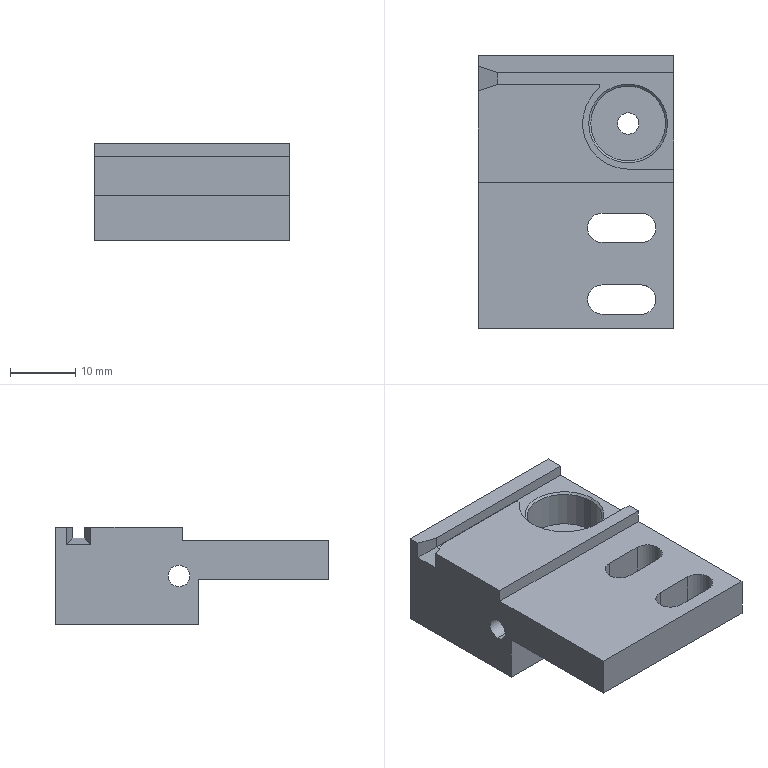Part | NX | features BREP 1 | 1 solid | 39 faces | box 30 x 42 x 15 mm | volume 11527 mm3 | plane 24 | cylinder 13 | cone 2 | commonest cylinder face diameters 4.5 x6 3.3 x4 11.5 x2 14 x1
STEP:
#1=CARTESIAN_POINT('',(-6.05,0.,5.8));
#2=VERTEX_POINT('',#1);
#3=CARTESIAN_POINT('',(-5.75,0.,5.5));
#4=VERTEX_POINT('',#3);
#5=CARTESIAN_POINT('',(-5.75,0.,5.5));
#6=DIRECTION('',(-0.7071,0.,0.7071));
#7=VECTOR('',#6,1000.);
#8=LINE('',#5,#7);
#9=EDGE_CURVE('',#2,#4,#8,.F.);
#10=ORIENTED_EDGE('',*,*,#9,.T.);
#11=CARTESIAN_POINT('',(5.75,0.,5.5));
#12=VERTEX_POINT('',#11);
#13=CARTESIAN_POINT('',(0.,0.,5.5));
#14=DIRECTION('',(0.,0.,1.));
#15=DIRECTION('',(1.,0.,0.));
#16=AXIS2_PLACEMENT_3D('',#13,#14,#15);
#17=CIRCLE('',#16,5.75);
#18=EDGE_CURVE('',#12,#4,#17,.T.);
#19=ORIENTED_EDGE('',*,*,#18,.F.);
#20=CARTESIAN_POINT('',(6.05,0.,5.8));
#21=VERTEX_POINT('',#20);
#22=CARTESIAN_POINT('',(5.75,0.,5.5));
#23=DIRECTION('',(0.7071,0.,0.7071));
#24=VECTOR('',#23,1000.);
#25=LINE('',#22,#24);
#26=EDGE_CURVE('',#21,#12,#25,.F.);
#27=ORIENTED_EDGE('',*,*,#26,.F.);
#28=CARTESIAN_POINT('',(0.,0.,5.8));
#29=DIRECTION('',(0.,0.,-1.));
#30=DIRECTION('',(1.,0.,0.));
#31=AXIS2_PLACEMENT_3D('',#28,#29,#30);
#32=CIRCLE('',#31,6.05);
#33=EDGE_CURVE('',#2,#21,#32,.T.);
#34=ORIENTED_EDGE('',*,*,#33,.F.);
#35=EDGE_LOOP('',(#10,#19,#27,#34));
#36=FACE_BOUND('',#35,.T.);
#37=CARTESIAN_POINT('',(0.,0.,5.5));
#38=DIRECTION('',(0.,0.,1.));
#39=DIRECTION('',(1.,0.,0.));
#40=AXIS2_PLACEMENT_3D('',#37,#38,#39);
#41=CONICAL_SURFACE('',#40,5.75,0.7854);
#42=ADVANCED_FACE('',(#36),#41,.F.);
#43=CARTESIAN_POINT('',(7.,-9.,7.5));
#44=VERTEX_POINT('',#43);
#45=CARTESIAN_POINT('',(-23.,-9.,7.5));
#46=VERTEX_POINT('',#45);
#47=CARTESIAN_POINT('',(-23.,-9.,7.5));
#48=DIRECTION('',(-1.,0.,0.));
#49=VECTOR('',#48,1000.);
#50=LINE('',#47,#49);
#51=EDGE_CURVE('',#44,#46,#50,.T.);
#52=ORIENTED_EDGE('',*,*,#51,.T.);
#53=CARTESIAN_POINT('',(-23.,-9.,5.5));
#54=VERTEX_POINT('',#53);
#55=CARTESIAN_POINT('',(-23.,-9.,5.5));
#56=DIRECTION('',(0.,0.,1.));
#57=VECTOR('',#56,1000.);
#58=LINE('',#55,#57);
#59=EDGE_CURVE('',#54,#46,#58,.T.);
#60=ORIENTED_EDGE('',*,*,#59,.F.);
#61=CARTESIAN_POINT('',(7.,-9.,5.5));
#62=VERTEX_POINT('',#61);
#63=CARTESIAN_POINT('',(-23.,-9.,5.5));
#64=DIRECTION('',(-1.,0.,0.));
#65=VECTOR('',#64,1000.);
#66=LINE('',#63,#65);
#67=EDGE_CURVE('',#62,#54,#66,.T.);
#68=ORIENTED_EDGE('',*,*,#67,.F.);
#69=CARTESIAN_POINT('',(7.,-9.,5.5));
#70=DIRECTION('',(0.,0.,1.));
#71=VECTOR('',#70,1000.);
#72=LINE('',#69,#71);
#73=EDGE_CURVE('',#62,#44,#72,.T.);
#74=ORIENTED_EDGE('',*,*,#73,.T.);
#75=EDGE_LOOP('',(#52,#60,#68,#74));
#76=FACE_BOUND('',#75,.T.);
#77=CARTESIAN_POINT('',(-23.,-9.,5.5));
#78=DIRECTION('',(0.,1.,0.));
#79=DIRECTION('',(0.,0.,1.));
#80=AXIS2_PLACEMENT_3D('',#77,#78,#79);
#81=PLANE('',#80);
#82=ADVANCED_FACE('',(#76),#81,.F.);
#83=CARTESIAN_POINT('',(-4.,-18.25,5.5));
#84=VERTEX_POINT('',#83);
#85=CARTESIAN_POINT('',(-4.,-13.75,5.5));
#86=VERTEX_POINT('',#85);
#87=CARTESIAN_POINT('',(-4.,-16.,5.5));
#88=DIRECTION('',(0.,0.,-1.));
#89=DIRECTION('',(1.,0.,0.));
#90=AXIS2_PLACEMENT_3D('',#87,#88,#89);
#91=CIRCLE('',#90,2.25);
#92=EDGE_CURVE('',#84,#86,#91,.T.);
#93=ORIENTED_EDGE('',*,*,#92,.T.);
#94=CARTESIAN_POINT('',(2.,-13.75,5.5));
#95=VERTEX_POINT('',#94);
#96=CARTESIAN_POINT('',(-4.,-13.75,5.5));
#97=DIRECTION('',(1.,0.,0.));
#98=VECTOR('',#97,1000.);
#99=LINE('',#96,#98);
#100=EDGE_CURVE('',#86,#95,#99,.T.);
#101=ORIENTED_EDGE('',*,*,#100,.T.);
#102=CARTESIAN_POINT('',(4.25,-16.,5.5));
#103=VERTEX_POINT('',#102);
#104=CARTESIAN_POINT('',(2.,-16.,5.5));
#105=DIRECTION('',(0.,0.,-1.));
#106=DIRECTION('',(1.,0.,0.));
#107=AXIS2_PLACEMENT_3D('',#104,#105,#106);
#108=CIRCLE('',#107,2.25);
#109=EDGE_CURVE('',#95,#103,#108,.T.);
#110=ORIENTED_EDGE('',*,*,#109,.T.);
#111=CARTESIAN_POINT('',(2.,-18.25,5.5));
#112=VERTEX_POINT('',#111);
#113=CARTESIAN_POINT('',(2.,-16.,5.5));
#114=DIRECTION('',(0.,0.,-1.));
#115=DIRECTION('',(1.,0.,0.));
#116=AXIS2_PLACEMENT_3D('',#113,#114,#115);
#117=CIRCLE('',#116,2.25);
#118=EDGE_CURVE('',#103,#112,#117,.T.);
#119=ORIENTED_EDGE('',*,*,#118,.T.);
#120=CARTESIAN_POINT('',(-4.,-18.25,5.5));
#121=DIRECTION('',(-1.,0.,0.));
#122=VECTOR('',#121,1000.);
#123=LINE('',#120,#122);
#124=EDGE_CURVE('',#112,#84,#123,.T.);
#125=ORIENTED_EDGE('',*,*,#124,.T.);
#126=EDGE_LOOP('',(#93,#101,#110,#119,#125));
#127=FACE_BOUND('',#126,.T.);
#128=CARTESIAN_POINT('',(7.,-31.5,5.5));
#129=VERTEX_POINT('',#128);
#130=CARTESIAN_POINT('',(7.,-9.,5.5));
#131=DIRECTION('',(0.,1.,0.));
#132=VECTOR('',#131,1000.);
#133=LINE('',#130,#132);
#134=EDGE_CURVE('',#129,#62,#133,.T.);
#135=ORIENTED_EDGE('',*,*,#134,.T.);
#136=ORIENTED_EDGE('',*,*,#67,.T.);
#137=CARTESIAN_POINT('',(-23.,-31.5,5.5));
#138=VERTEX_POINT('',#137);
#139=CARTESIAN_POINT('',(-23.,-9.,5.5));
#140=DIRECTION('',(0.,-1.,0.));
#141=VECTOR('',#140,1000.);
#142=LINE('',#139,#141);
#143=EDGE_CURVE('',#54,#138,#142,.T.);
#144=ORIENTED_EDGE('',*,*,#143,.T.);
#145=CARTESIAN_POINT('',(-23.,-31.5,5.5));
#146=DIRECTION('',(1.,0.,0.));
#147=VECTOR('',#146,1000.);
#148=LINE('',#145,#147);
#149=EDGE_CURVE('',#138,#129,#148,.T.);
#150=ORIENTED_EDGE('',*,*,#149,.T.);
#151=EDGE_LOOP('',(#135,#136,#144,#150));
#152=FACE_BOUND('',#151,.T.);
#153=CARTESIAN_POINT('',(-4.,-29.25,5.5));
#154=VERTEX_POINT('',#153);
#155=CARTESIAN_POINT('',(-4.,-24.75,5.5));
#156=VERTEX_POINT('',#155);
#157=CARTESIAN_POINT('',(-4.,-27.,5.5));
#158=DIRECTION('',(0.,0.,-1.));
#159=DIRECTION('',(1.,0.,0.));
#160=AXIS2_PLACEMENT_3D('',#157,#158,#159);
#161=CIRCLE('',#160,2.25);
#162=EDGE_CURVE('',#154,#156,#161,.T.);
#163=ORIENTED_EDGE('',*,*,#162,.T.);
#164=CARTESIAN_POINT('',(2.,-24.75,5.5));
#165=VERTEX_POINT('',#164);
#166=CARTESIAN_POINT('',(-4.,-24.75,5.5));
#167=DIRECTION('',(1.,0.,0.));
#168=VECTOR('',#167,1000.);
#169=LINE('',#166,#168);
#170=EDGE_CURVE('',#156,#165,#169,.T.);
#171=ORIENTED_EDGE('',*,*,#170,.T.);
#172=CARTESIAN_POINT('',(4.25,-27.,5.5));
#173=VERTEX_POINT('',#172);
#174=CARTESIAN_POINT('',(2.,-27.,5.5));
#175=DIRECTION('',(0.,0.,-1.));
#176=DIRECTION('',(1.,0.,0.));
#177=AXIS2_PLACEMENT_3D('',#174,#175,#176);
#178=CIRCLE('',#177,2.25);
#179=EDGE_CURVE('',#165,#173,#178,.T.);
#180=ORIENTED_EDGE('',*,*,#179,.T.);
#181=CARTESIAN_POINT('',(2.,-29.25,5.5));
#182=VERTEX_POINT('',#181);
#183=CARTESIAN_POINT('',(2.,-27.,5.5));
#184=DIRECTION('',(0.,0.,-1.));
#185=DIRECTION('',(1.,0.,0.));
#186=AXIS2_PLACEMENT_3D('',#183,#184,#185);
#187=CIRCLE('',#186,2.25);
#188=EDGE_CURVE('',#173,#182,#187,.T.);
#189=ORIENTED_EDGE('',*,*,#188,.T.);
#190=CARTESIAN_POINT('',(-4.,-29.25,5.5));
#191=DIRECTION('',(-1.,0.,0.));
#192=VECTOR('',#191,1000.);
#193=LINE('',#190,#192);
#194=EDGE_CURVE('',#182,#154,#193,.T.);
#195=ORIENTED_EDGE('',*,*,#194,.T.);
#196=EDGE_LOOP('',(#163,#171,#180,#189,#195));
#197=FACE_BOUND('',#196,.T.);
#198=CARTESIAN_POINT('',(0.,0.,5.5));
#199=DIRECTION('',(0.,0.,1.));
#200=DIRECTION('',(1.,0.,0.));
#201=AXIS2_PLACEMENT_3D('',#198,#199,#200);
#202=PLANE('',#201);
#203=ADVANCED_FACE('',(#127,#152,#197),#202,.T.);
#204=CARTESIAN_POINT('',(-23.,-8.5,-1.65));
#205=VERTEX_POINT('',#204);
#206=CARTESIAN_POINT('',(7.,-8.5,-1.65));
#207=VERTEX_POINT('',#206);
#208=CARTESIAN_POINT('',(-23.,-8.5,-1.65));
#209=DIRECTION('',(-1.,0.,0.));
#210=VECTOR('',#209,1000.);
#211=LINE('',#208,#210);
#212=EDGE_CURVE('',#205,#207,#211,.F.);
#213=ORIENTED_EDGE('',*,*,#212,.T.);
#214=CARTESIAN_POINT('',(7.,-8.5,1.65));
#215=VERTEX_POINT('',#214);
#216=CARTESIAN_POINT('',(7.,-8.5,0.));
#217=DIRECTION('',(-1.,0.,0.));
#218=DIRECTION('',(0.,0.,1.));
#219=AXIS2_PLACEMENT_3D('',#216,#217,#218);
#220=CIRCLE('',#219,1.65);
#221=EDGE_CURVE('',#215,#207,#220,.T.);
#222=ORIENTED_EDGE('',*,*,#221,.F.);
#223=CARTESIAN_POINT('',(-23.,-8.5,1.65));
#224=VERTEX_POINT('',#223);
#225=CARTESIAN_POINT('',(-23.,-8.5,1.65));
#226=DIRECTION('',(-1.,0.,0.));
#227=VECTOR('',#226,1000.);
#228=LINE('',#225,#227);
#229=EDGE_CURVE('',#224,#215,#228,.F.);
#230=ORIENTED_EDGE('',*,*,#229,.F.);
#231=CARTESIAN_POINT('',(-23.,-8.5,0.));
#232=DIRECTION('',(-1.,0.,0.));
#233=DIRECTION('',(0.,0.,1.));
#234=AXIS2_PLACEMENT_3D('',#231,#232,#233);
#235=CIRCLE('',#234,1.65);
#236=EDGE_CURVE('',#224,#205,#235,.T.);
#237=ORIENTED_EDGE('',*,*,#236,.T.);
#238=EDGE_LOOP('',(#213,#222,#230,#237));
#239=FACE_BOUND('',#238,.T.);
#240=CARTESIAN_POINT('',(-23.,-8.5,0.));
#241=DIRECTION('',(-1.,0.,0.));
#242=DIRECTION('',(0.,0.,1.));
#243=AXIS2_PLACEMENT_3D('',#240,#241,#242);
#244=CYLINDRICAL_SURFACE('',#243,1.65);
#245=ADVANCED_FACE('',(#239),#244,.F.);
#246=CARTESIAN_POINT('',(-4.33,5.5,5.8));
#247=VERTEX_POINT('',#246);
#248=CARTESIAN_POINT('',(-4.33,6.,5.8));
#249=VERTEX_POINT('',#248);
#250=CARTESIAN_POINT('',(-4.33,6.,5.8));
#251=DIRECTION('',(0.,1.,0.));
#252=VECTOR('',#251,1000.);
#253=LINE('',#250,#252);
#254=EDGE_CURVE('',#247,#249,#253,.T.);
#255=ORIENTED_EDGE('',*,*,#254,.T.);
#256=CARTESIAN_POINT('',(-4.33,6.,7.5));
#257=VERTEX_POINT('',#256);
#258=CARTESIAN_POINT('',(-4.33,6.,4.92));
#259=DIRECTION('',(0.,0.,1.));
#260=VECTOR('',#259,1000.);
#261=LINE('',#258,#260);
#262=EDGE_CURVE('',#249,#257,#261,.T.);
#263=ORIENTED_EDGE('',*,*,#262,.T.);
#264=CARTESIAN_POINT('',(-4.33,5.5,7.5));
#265=VERTEX_POINT('',#264);
#266=CARTESIAN_POINT('',(-4.33,6.,7.5));
#267=DIRECTION('',(0.,-1.,0.));
#268=VECTOR('',#267,1000.);
#269=LINE('',#266,#268);
#270=EDGE_CURVE('',#257,#265,#269,.T.);
#271=ORIENTED_EDGE('',*,*,#270,.T.);
#272=CARTESIAN_POINT('',(-4.33,5.5,4.92));
#273=DIRECTION('',(0.,0.,1.));
#274=VECTOR('',#273,1000.);
#275=LINE('',#272,#274);
#276=EDGE_CURVE('',#247,#265,#275,.T.);
#277=ORIENTED_EDGE('',*,*,#276,.F.);
#278=EDGE_LOOP('',(#255,#263,#271,#277));
#279=FACE_BOUND('',#278,.T.);
#280=CARTESIAN_POINT('',(-4.33,6.,4.92));
#281=DIRECTION('',(-1.,0.,0.));
#282=DIRECTION('',(0.,0.,1.));
#283=AXIS2_PLACEMENT_3D('',#280,#281,#282);
#284=PLANE('',#283);
#285=ADVANCED_FACE('',(#279),#284,.F.);
#286=CARTESIAN_POINT('',(-20.,6.,5.8));
#287=VERTEX_POINT('',#286);
#288=CARTESIAN_POINT('',(-23.,5.,4.8));
#289=VERTEX_POINT('',#288);
#290=CARTESIAN_POINT('',(-20.,6.,5.8));
#291=DIRECTION('',(-0.9045,-0.3015,-0.3015));
#292=VECTOR('',#291,1000.);
#293=LINE('',#290,#292);
#294=EDGE_CURVE('',#287,#289,#293,.T.);
#295=ORIENTED_EDGE('',*,*,#294,.T.);
#296=CARTESIAN_POINT('',(-23.,5.,7.5));
#297=VERTEX_POINT('',#296);
#298=CARTESIAN_POINT('',(-23.,5.,7.5));
#299=DIRECTION('',(0.,0.,-1.));
#300=VECTOR('',#299,1000.);
#301=LINE('',#298,#300);
#302=EDGE_CURVE('',#297,#289,#301,.T.);
#303=ORIENTED_EDGE('',*,*,#302,.F.);
#304=CARTESIAN_POINT('',(-20.,6.,7.5));
#305=VERTEX_POINT('',#304);
#306=CARTESIAN_POINT('',(-20.,6.,7.5));
#307=DIRECTION('',(-0.9487,-0.3162,0.));
#308=VECTOR('',#307,1000.);
#309=LINE('',#306,#308);
#310=EDGE_CURVE('',#305,#297,#309,.T.);
#311=ORIENTED_EDGE('',*,*,#310,.F.);
#312=CARTESIAN_POINT('',(-20.,6.,5.8));
#313=DIRECTION('',(0.,0.,1.));
#314=VECTOR('',#313,1000.);
#315=LINE('',#312,#314);
#316=EDGE_CURVE('',#287,#305,#315,.T.);
#317=ORIENTED_EDGE('',*,*,#316,.F.);
#318=EDGE_LOOP('',(#295,#303,#311,#317));
#319=FACE_BOUND('',#318,.T.);
#320=CARTESIAN_POINT('',(-20.,6.,5.8));
#321=DIRECTION('',(0.3162,-0.9487,0.));
#322=DIRECTION('',(0.,0.,1.));
#323=AXIS2_PLACEMENT_3D('',#320,#321,#322);
#324=PLANE('',#323);
#325=ADVANCED_FACE('',(#319),#324,.F.);
#326=CARTESIAN_POINT('',(-20.,7.8,5.8));
#327=VERTEX_POINT('',#326);
#328=CARTESIAN_POINT('',(-23.,8.8,4.8));
#329=VERTEX_POINT('',#328);
#330=CARTESIAN_POINT('',(-17.873,7.091,6.509));
#331=DIRECTION('',(-0.9045,0.3015,-0.3015));
#332=VECTOR('',#331,1000.);
#333=LINE('',#330,#332);
#334=EDGE_CURVE('',#327,#329,#333,.T.);
#335=ORIENTED_EDGE('',*,*,#334,.T.);
#336=CARTESIAN_POINT('',(-23.,7.8,4.8));
#337=DIRECTION('',(0.,1.,0.));
#338=VECTOR('',#337,1000.);
#339=LINE('',#336,#338);
#340=EDGE_CURVE('',#289,#329,#339,.T.);
#341=ORIENTED_EDGE('',*,*,#340,.F.);
#342=ORIENTED_EDGE('',*,*,#294,.F.);
#343=CARTESIAN_POINT('',(-20.,6.,5.8));
#344=DIRECTION('',(0.,-1.,0.));
#345=VECTOR('',#344,1000.);
#346=LINE('',#343,#345);
#347=EDGE_CURVE('',#327,#287,#346,.T.);
#348=ORIENTED_EDGE('',*,*,#347,.F.);
#349=EDGE_LOOP('',(#335,#341,#342,#348));
#350=FACE_BOUND('',#349,.T.);
#351=CARTESIAN_POINT('',(-20.,0.,5.8));
#352=DIRECTION('',(-0.3162,0.,0.9487));
#353=DIRECTION('',(0.,1.,0.));
#354=AXIS2_PLACEMENT_3D('',#351,#352,#353);
#355=PLANE('',#354);
#356=ADVANCED_FACE('',(#350),#355,.T.);
#357=CARTESIAN_POINT('',(-23.,8.8,7.5));
#358=VERTEX_POINT('',#357);
#359=CARTESIAN_POINT('',(-20.,7.8,7.5));
#360=VERTEX_POINT('',#359);
#361=CARTESIAN_POINT('',(-23.,8.8,7.5));
#362=DIRECTION('',(0.9487,-0.3162,0.));
#363=VECTOR('',#362,1000.);
#364=LINE('',#361,#363);
#365=EDGE_CURVE('',#358,#360,#364,.T.);
#366=ORIENTED_EDGE('',*,*,#365,.F.);
#367=CARTESIAN_POINT('',(-23.,8.8,7.5));
#368=DIRECTION('',(0.,0.,1.));
#369=VECTOR('',#368,1000.);
#370=LINE('',#367,#369);
#371=EDGE_CURVE('',#329,#358,#370,.T.);
#372=ORIENTED_EDGE('',*,*,#371,.F.);
#373=ORIENTED_EDGE('',*,*,#334,.F.);
#374=CARTESIAN_POINT('',(-20.,7.8,5.8));
#375=DIRECTION('',(0.,0.,-1.));
#376=VECTOR('',#375,1000.);
#377=LINE('',#374,#376);
#378=EDGE_CURVE('',#360,#327,#377,.T.);
#379=ORIENTED_EDGE('',*,*,#378,.F.);
#380=EDGE_LOOP('',(#366,#372,#373,#379));
#381=FACE_BOUND('',#380,.T.);
#382=CARTESIAN_POINT('',(-23.,8.8,7.5));
#383=DIRECTION('',(0.3162,0.9487,0.));
#384=DIRECTION('',(0.,0.,1.));
#385=AXIS2_PLACEMENT_3D('',#382,#383,#384);
#386=PLANE('',#385);
#387=ADVANCED_FACE('',(#381),#386,.F.);
#388=CARTESIAN_POINT('',(0.,-7.,5.8));
#389=VERTEX_POINT('',#388);
#390=CARTESIAN_POINT('',(0.,0.,5.8));
#391=DIRECTION('',(0.,0.,-1.));
#392=DIRECTION('',(1.,0.,0.));
#393=AXIS2_PLACEMENT_3D('',#390,#391,#392);
#394=CIRCLE('',#393,7.);
#395=EDGE_CURVE('',#389,#247,#394,.T.);
#396=ORIENTED_EDGE('',*,*,#395,.T.);
#397=ORIENTED_EDGE('',*,*,#276,.T.);
#398=CARTESIAN_POINT('',(0.,-7.,7.5));
#399=VERTEX_POINT('',#398);
#400=CARTESIAN_POINT('',(0.,0.,7.5));
#401=DIRECTION('',(0.,0.,1.));
#402=DIRECTION('',(1.,0.,0.));
#403=AXIS2_PLACEMENT_3D('',#400,#401,#402);
#404=CIRCLE('',#403,7.);
#405=EDGE_CURVE('',#265,#399,#404,.T.);
#406=ORIENTED_EDGE('',*,*,#405,.T.);
#407=CARTESIAN_POINT('',(0.,-7.,-17.743));
#408=DIRECTION('',(0.,0.,1.));
#409=VECTOR('',#408,1000.);
#410=LINE('',#407,#409);
#411=EDGE_CURVE('',#389,#399,#410,.T.);
#412=ORIENTED_EDGE('',*,*,#411,.F.);
#413=EDGE_LOOP('',(#396,#397,#406,#412));
#414=FACE_BOUND('',#413,.T.);
#415=CARTESIAN_POINT('',(0.,0.,-17.743));
#416=DIRECTION('',(0.,0.,1.));
#417=DIRECTION('',(1.,0.,0.));
#418=AXIS2_PLACEMENT_3D('',#415,#416,#417);
#419=CYLINDRICAL_SURFACE('',#418,7.);
#420=ADVANCED_FACE('',(#414),#419,.F.);
#421=CARTESIAN_POINT('',(7.,-7.,5.8));
#422=VERTEX_POINT('',#421);
#423=CARTESIAN_POINT('',(0.,-7.,5.8));
#424=DIRECTION('',(-1.,0.,0.));
#425=VECTOR('',#424,1000.);
#426=LINE('',#423,#425);
#427=EDGE_CURVE('',#422,#389,#426,.T.);
#428=ORIENTED_EDGE('',*,*,#427,.T.);
#429=ORIENTED_EDGE('',*,*,#411,.T.);
#430=CARTESIAN_POINT('',(7.,-7.,7.5));
#431=VERTEX_POINT('',#430);
#432=CARTESIAN_POINT('',(0.,-7.,7.5));
#433=DIRECTION('',(1.,0.,0.));
#434=VECTOR('',#433,1000.);
#435=LINE('',#432,#434);
#436=EDGE_CURVE('',#399,#431,#435,.T.);
#437=ORIENTED_EDGE('',*,*,#436,.T.);
#438=CARTESIAN_POINT('',(7.,-7.,7.5));
#439=DIRECTION('',(0.,0.,1.));
#440=VECTOR('',#439,1000.);
#441=LINE('',#438,#440);
#442=EDGE_CURVE('',#422,#431,#441,.T.);
#443=ORIENTED_EDGE('',*,*,#442,.F.);
#444=EDGE_LOOP('',(#428,#429,#437,#443));
#445=FACE_BOUND('',#444,.T.);
#446=CARTESIAN_POINT('',(0.,-7.,-17.743));
#447=DIRECTION('',(0.,-1.,0.));
#448=DIRECTION('',(0.,0.,-1.));
#449=AXIS2_PLACEMENT_3D('',#446,#447,#448);
#450=PLANE('',#449);
#451=ADVANCED_FACE('',(#445),#450,.F.);
#452=CARTESIAN_POINT('',(7.,7.8,5.8));
#453=VERTEX_POINT('',#452);
#454=CARTESIAN_POINT('',(-23.,7.8,5.8));
#455=DIRECTION('',(-1.,0.,0.));
#456=VECTOR('',#455,1000.);
#457=LINE('',#454,#456);
#458=EDGE_CURVE('',#453,#327,#457,.T.);
#459=ORIENTED_EDGE('',*,*,#458,.T.);
#460=ORIENTED_EDGE('',*,*,#347,.T.);
#461=CARTESIAN_POINT('',(-23.,6.,5.8));
#462=DIRECTION('',(1.,0.,0.));
#463=VECTOR('',#462,1000.);
#464=LINE('',#461,#463);
#465=EDGE_CURVE('',#287,#249,#464,.T.);
#466=ORIENTED_EDGE('',*,*,#465,.T.);
#467=ORIENTED_EDGE('',*,*,#254,.F.);
#468=ORIENTED_EDGE('',*,*,#395,.F.);
#469=ORIENTED_EDGE('',*,*,#427,.F.);
#470=CARTESIAN_POINT('',(7.,7.8,5.8));
#471=DIRECTION('',(0.,1.,0.));
#472=VECTOR('',#471,1000.);
#473=LINE('',#470,#472);
#474=EDGE_CURVE('',#422,#453,#473,.T.);
#475=ORIENTED_EDGE('',*,*,#474,.T.);
#476=EDGE_LOOP('',(#459,#460,#466,#467,#468,#469,#475));
#477=FACE_BOUND('',#476,.T.);
#478=CARTESIAN_POINT('',(0.,0.,5.8));
#479=DIRECTION('',(0.,0.,-1.));
#480=DIRECTION('',(1.,0.,0.));
#481=AXIS2_PLACEMENT_3D('',#478,#479,#480);
#482=CIRCLE('',#481,6.05);
#483=EDGE_CURVE('',#21,#2,#482,.T.);
#484=ORIENTED_EDGE('',*,*,#483,.T.);
#485=ORIENTED_EDGE('',*,*,#33,.T.);
#486=EDGE_LOOP('',(#484,#485));
#487=FACE_BOUND('',#486,.T.);
#488=CARTESIAN_POINT('',(0.,0.,5.8));
#489=DIRECTION('',(0.,0.,1.));
#490=DIRECTION('',(1.,0.,0.));
#491=AXIS2_PLACEMENT_3D('',#488,#489,#490);
#492=PLANE('',#491);
#493=ADVANCED_FACE('',(#477,#487),#492,.T.);
#494=CARTESIAN_POINT('',(-23.,6.,7.5));
#495=DIRECTION('',(1.,0.,0.));
#496=VECTOR('',#495,1000.);
#497=LINE('',#494,#496);
#498=EDGE_CURVE('',#305,#257,#497,.T.);
#499=ORIENTED_EDGE('',*,*,#498,.T.);
#500=ORIENTED_EDGE('',*,*,#262,.F.);
#501=ORIENTED_EDGE('',*,*,#465,.F.);
#502=ORIENTED_EDGE('',*,*,#316,.T.);
#503=EDGE_LOOP('',(#499,#500,#501,#502));
#504=FACE_BOUND('',#503,.T.);
#505=CARTESIAN_POINT('',(-23.,6.,5.8));
#506=DIRECTION('',(0.,-1.,0.));
#507=DIRECTION('',(1.,0.,0.));
#508=AXIS2_PLACEMENT_3D('',#505,#506,#507);
#509=PLANE('',#508);
#510=ADVANCED_FACE('',(#504),#509,.F.);
#511=CARTESIAN_POINT('',(7.,7.8,7.5));
#512=VERTEX_POINT('',#511);
#513=CARTESIAN_POINT('',(-23.,7.8,7.5));
#514=DIRECTION('',(-1.,0.,0.));
#515=VECTOR('',#514,1000.);
#516=LINE('',#513,#515);
#517=EDGE_CURVE('',#512,#360,#516,.T.);
#518=ORIENTED_EDGE('',*,*,#517,.T.);
#519=ORIENTED_EDGE('',*,*,#378,.T.);
#520=ORIENTED_EDGE('',*,*,#458,.F.);
#521=CARTESIAN_POINT('',(7.,7.8,5.8));
#522=DIRECTION('',(0.,0.,1.));
#523=VECTOR('',#522,1000.);
#524=LINE('',#521,#523);
#525=EDGE_CURVE('',#453,#512,#524,.T.);
#526=ORIENTED_EDGE('',*,*,#525,.T.);
#527=EDGE_LOOP('',(#518,#519,#520,#526));
#528=FACE_BOUND('',#527,.T.);
#529=CARTESIAN_POINT('',(-23.,7.8,5.8));
#530=DIRECTION('',(0.,1.,0.));
#531=DIRECTION('',(-1.,0.,0.));
#532=AXIS2_PLACEMENT_3D('',#529,#530,#531);
#533=PLANE('',#532);
#534=ADVANCED_FACE('',(#528),#533,.F.);
#535=CARTESIAN_POINT('',(-1.65,0.,0.));
#536=VERTEX_POINT('',#535);
#537=CARTESIAN_POINT('',(-1.65,0.,-7.5));
#538=VERTEX_POINT('',#537);
#539=CARTESIAN_POINT('',(-1.65,0.,0.));
#540=DIRECTION('',(0.,0.,1.));
#541=VECTOR('',#540,1000.);
#542=LINE('',#539,#541);
#543=EDGE_CURVE('',#536,#538,#542,.F.);
#544=ORIENTED_EDGE('',*,*,#543,.T.);
#545=CARTESIAN_POINT('',(1.65,0.,-7.5));
#546=VERTEX_POINT('',#545);
#547=CARTESIAN_POINT('',(0.,0.,-7.5));
#548=DIRECTION('',(0.,0.,1.));
#549=DIRECTION('',(1.,0.,0.));
#550=AXIS2_PLACEMENT_3D('',#547,#548,#549);
#551=CIRCLE('',#550,1.65);
#552=EDGE_CURVE('',#546,#538,#551,.T.);
#553=ORIENTED_EDGE('',*,*,#552,.F.);
#554=CARTESIAN_POINT('',(1.65,0.,0.));
#555=VERTEX_POINT('',#554);
#556=CARTESIAN_POINT('',(1.65,0.,0.));
#557=DIRECTION('',(0.,0.,1.));
#558=VECTOR('',#557,1000.);
#559=LINE('',#556,#558);
#560=EDGE_CURVE('',#555,#546,#559,.F.);
#561=ORIENTED_EDGE('',*,*,#560,.F.);
#562=CARTESIAN_POINT('',(0.,0.,0.));
#563=DIRECTION('',(0.,0.,1.));
#564=DIRECTION('',(1.,0.,0.));
#565=AXIS2_PLACEMENT_3D('',#562,#563,#564);
#566=CIRCLE('',#565,1.65);
#567=EDGE_CURVE('',#555,#536,#566,.T.);
#568=ORIENTED_EDGE('',*,*,#567,.T.);
#569=EDGE_LOOP('',(#544,#553,#561,#568));
#570=FACE_BOUND('',#569,.T.);
#571=CARTESIAN_POINT('',(0.,0.,0.));
#572=DIRECTION('',(0.,0.,1.));
#573=DIRECTION('',(1.,0.,0.));
#574=AXIS2_PLACEMENT_3D('',#571,#572,#573);
#575=CYLINDRICAL_SURFACE('',#574,1.65);
#576=ADVANCED_FACE('',(#570),#575,.F.);
#577=CARTESIAN_POINT('',(-5.75,0.,0.));
#578=VERTEX_POINT('',#577);
#579=CARTESIAN_POINT('',(5.75,0.,0.));
#580=VERTEX_POINT('',#579);
#581=CARTESIAN_POINT('',(0.,0.,0.));
#582=DIRECTION('',(0.,0.,-1.));
#583=DIRECTION('',(-1.,0.,0.));
#584=AXIS2_PLACEMENT_3D('',#581,#582,#583);
#585=CIRCLE('',#584,5.75);
#586=EDGE_CURVE('',#578,#580,#585,.T.);
#587=ORIENTED_EDGE('',*,*,#586,.F.);
#588=CARTESIAN_POINT('',(0.,0.,0.));
#589=DIRECTION('',(0.,0.,-1.));
#590=DIRECTION('',(-1.,0.,0.));
#591=AXIS2_PLACEMENT_3D('',#588,#589,#590);
#592=CIRCLE('',#591,5.75);
#593=EDGE_CURVE('',#580,#578,#592,.T.);
#594=ORIENTED_EDGE('',*,*,#593,.F.);
#595=EDGE_LOOP('',(#587,#594));
#596=FACE_BOUND('',#595,.T.);
#597=ORIENTED_EDGE('',*,*,#567,.F.);
#598=CARTESIAN_POINT('',(0.,0.,0.));
#599=DIRECTION('',(0.,0.,1.));
#600=DIRECTION('',(1.,0.,0.));
#601=AXIS2_PLACEMENT_3D('',#598,#599,#600);
#602=CIRCLE('',#601,1.65);
#603=EDGE_CURVE('',#536,#555,#602,.T.);
#604=ORIENTED_EDGE('',*,*,#603,.F.);
#605=EDGE_LOOP('',(#597,#604));
#606=FACE_BOUND('',#605,.T.);
#607=CARTESIAN_POINT('',(0.,0.,0.));
#608=DIRECTION('',(0.,0.,-1.));
#609=DIRECTION('',(-1.,0.,0.));
#610=AXIS2_PLACEMENT_3D('',#607,#608,#609);
#611=PLANE('',#610);
#612=ADVANCED_FACE('',(#596,#606),#611,.F.);
#613=CARTESIAN_POINT('',(7.,-31.5,-0.5));
#614=VERTEX_POINT('',#613);
#615=CARTESIAN_POINT('',(-23.,-31.5,-0.5));
#616=VERTEX_POINT('',#615);
#617=CARTESIAN_POINT('',(10.,-31.5,-0.5));
#618=DIRECTION('',(-1.,0.,0.));
#619=VECTOR('',#618,1000.);
#620=LINE('',#617,#619);
#621=EDGE_CURVE('',#614,#616,#620,.T.);
#622=ORIENTED_EDGE('',*,*,#621,.T.);
#623=CARTESIAN_POINT('',(-23.,-11.5,-0.5));
#624=VERTEX_POINT('',#623);
#625=CARTESIAN_POINT('',(-23.,-31.5,-0.5));
#626=DIRECTION('',(0.,1.,0.));
#627=VECTOR('',#626,1000.);
#628=LINE('',#625,#627);
#629=EDGE_CURVE('',#616,#624,#628,.T.);
#630=ORIENTED_EDGE('',*,*,#629,.T.);
#631=CARTESIAN_POINT('',(7.,-11.5,-0.5));
#632=VERTEX_POINT('',#631);
#633=CARTESIAN_POINT('',(10.,-11.5,-0.5));
#634=DIRECTION('',(-1.,0.,0.));
#635=VECTOR('',#634,1000.);
#636=LINE('',#633,#635);
#637=EDGE_CURVE('',#632,#624,#636,.T.);
#638=ORIENTED_EDGE('',*,*,#637,.F.);
#639=CARTESIAN_POINT('',(7.,10.5,-0.5));
#640=DIRECTION('',(0.,1.,0.));
#641=VECTOR('',#640,1000.);
#642=LINE('',#639,#641);
#643=EDGE_CURVE('',#614,#632,#642,.T.);
#644=ORIENTED_EDGE('',*,*,#643,.F.);
#645=EDGE_LOOP('',(#622,#630,#638,#644));
#646=FACE_BOUND('',#645,.T.);
#647=CARTESIAN_POINT('',(2.,-13.75,-0.5));
#648=VERTEX_POINT('',#647);
#649=CARTESIAN_POINT('',(-4.,-13.75,-0.5));
#650=VERTEX_POINT('',#649);
#651=CARTESIAN_POINT('',(10.,-13.75,-0.5));
#652=DIRECTION('',(-1.,0.,0.));
#653=VECTOR('',#652,1000.);
#654=LINE('',#651,#653);
#655=EDGE_CURVE('',#648,#650,#654,.T.);
#656=ORIENTED_EDGE('',*,*,#655,.T.);
#657=CARTESIAN_POINT('',(-4.,-18.25,-0.5));
#658=VERTEX_POINT('',#657);
#659=CARTESIAN_POINT('',(-4.,-16.,-0.5));
#660=DIRECTION('',(0.,0.,1.));
#661=DIRECTION('',(1.,0.,0.));
#662=AXIS2_PLACEMENT_3D('',#659,#660,#661);
#663=CIRCLE('',#662,2.25);
#664=EDGE_CURVE('',#650,#658,#663,.T.);
#665=ORIENTED_EDGE('',*,*,#664,.T.);
#666=CARTESIAN_POINT('',(2.,-18.25,-0.5));
#667=VERTEX_POINT('',#666);
#668=CARTESIAN_POINT('',(10.,-18.25,-0.5));
#669=DIRECTION('',(1.,0.,0.));
#670=VECTOR('',#669,1000.);
#671=LINE('',#668,#670);
#672=EDGE_CURVE('',#658,#667,#671,.T.);
#673=ORIENTED_EDGE('',*,*,#672,.T.);
#674=CARTESIAN_POINT('',(4.25,-16.,-0.5));
#675=VERTEX_POINT('',#674);
#676=CARTESIAN_POINT('',(2.,-16.,-0.5));
#677=DIRECTION('',(0.,0.,1.));
#678=DIRECTION('',(1.,0.,0.));
#679=AXIS2_PLACEMENT_3D('',#676,#677,#678);
#680=CIRCLE('',#679,2.25);
#681=EDGE_CURVE('',#667,#675,#680,.T.);
#682=ORIENTED_EDGE('',*,*,#681,.T.);
#683=CARTESIAN_POINT('',(2.,-16.,-0.5));
#684=DIRECTION('',(0.,0.,1.));
#685=DIRECTION('',(1.,0.,0.));
#686=AXIS2_PLACEMENT_3D('',#683,#684,#685);
#687=CIRCLE('',#686,2.25);
#688=EDGE_CURVE('',#675,#648,#687,.T.);
#689=ORIENTED_EDGE('',*,*,#688,.T.);
#690=EDGE_LOOP('',(#656,#665,#673,#682,#689));
#691=FACE_BOUND('',#690,.T.);
#692=CARTESIAN_POINT('',(2.,-24.75,-0.5));
#693=VERTEX_POINT('',#692);
#694=CARTESIAN_POINT('',(-4.,-24.75,-0.5));
#695=VERTEX_POINT('',#694);
#696=CARTESIAN_POINT('',(10.,-24.75,-0.5));
#697=DIRECTION('',(-1.,0.,0.));
#698=VECTOR('',#697,1000.);
#699=LINE('',#696,#698);
#700=EDGE_CURVE('',#693,#695,#699,.T.);
#701=ORIENTED_EDGE('',*,*,#700,.T.);
#702=CARTESIAN_POINT('',(-4.,-29.25,-0.5));
#703=VERTEX_POINT('',#702);
#704=CARTESIAN_POINT('',(-4.,-27.,-0.5));
#705=DIRECTION('',(0.,0.,1.));
#706=DIRECTION('',(1.,0.,0.));
#707=AXIS2_PLACEMENT_3D('',#704,#705,#706);
#708=CIRCLE('',#707,2.25);
#709=EDGE_CURVE('',#695,#703,#708,.T.);
#710=ORIENTED_EDGE('',*,*,#709,.T.);
#711=CARTESIAN_POINT('',(2.,-29.25,-0.5));
#712=VERTEX_POINT('',#711);
#713=CARTESIAN_POINT('',(10.,-29.25,-0.5));
#714=DIRECTION('',(1.,0.,0.));
#715=VECTOR('',#714,1000.);
#716=LINE('',#713,#715);
#717=EDGE_CURVE('',#703,#712,#716,.T.);
#718=ORIENTED_EDGE('',*,*,#717,.T.);
#719=CARTESIAN_POINT('',(4.25,-27.,-0.5));
#720=VERTEX_POINT('',#719);
#721=CARTESIAN_POINT('',(2.,-27.,-0.5));
#722=DIRECTION('',(0.,0.,1.));
#723=DIRECTION('',(1.,0.,0.));
#724=AXIS2_PLACEMENT_3D('',#721,#722,#723);
#725=CIRCLE('',#724,2.25);
#726=EDGE_CURVE('',#712,#720,#725,.T.);
#727=ORIENTED_EDGE('',*,*,#726,.T.);
#728=CARTESIAN_POINT('',(2.,-27.,-0.5));
#729=DIRECTION('',(0.,0.,1.));
#730=DIRECTION('',(1.,0.,0.));
#731=AXIS2_PLACEMENT_3D('',#728,#729,#730);
#732=CIRCLE('',#731,2.25);
#733=EDGE_CURVE('',#720,#693,#732,.T.);
#734=ORIENTED_EDGE('',*,*,#733,.T.);
#735=EDGE_LOOP('',(#701,#710,#718,#727,#734));
#736=FACE_BOUND('',#735,.T.);
#737=CARTESIAN_POINT('',(10.,-31.5,-0.5));
#738=DIRECTION('',(0.,0.,1.));
#739=DIRECTION('',(1.,0.,0.));
#740=AXIS2_PLACEMENT_3D('',#737,#738,#739);
#741=PLANE('',#740);
#742=ADVANCED_FACE('',(#646,#691,#736),#741,.F.);
#743=ORIENTED_EDGE('',*,*,#637,.T.);
#744=CARTESIAN_POINT('',(-23.,-11.5,-7.5));
#745=VERTEX_POINT('',#744);
#746=CARTESIAN_POINT('',(-23.,-11.5,-7.5));
#747=DIRECTION('',(0.,0.,-1.));
#748=VECTOR('',#747,1000.);
#749=LINE('',#746,#748);
#750=EDGE_CURVE('',#624,#745,#749,.T.);
#751=ORIENTED_EDGE('',*,*,#750,.T.);
#752=CARTESIAN_POINT('',(7.,-11.5,-7.5));
#753=VERTEX_POINT('',#752);
#754=CARTESIAN_POINT('',(10.,-11.5,-7.5));
#755=DIRECTION('',(-1.,0.,0.));
#756=VECTOR('',#755,1000.);
#757=LINE('',#754,#756);
#758=EDGE_CURVE('',#753,#745,#757,.T.);
#759=ORIENTED_EDGE('',*,*,#758,.F.);
#760=CARTESIAN_POINT('',(7.,-11.5,7.5));
#761=DIRECTION('',(0.,0.,-1.));
#762=VECTOR('',#761,1000.);
#763=LINE('',#760,#762);
#764=EDGE_CURVE('',#632,#753,#763,.T.);
#765=ORIENTED_EDGE('',*,*,#764,.F.);
#766=EDGE_LOOP('',(#743,#751,#759,#765));
#767=FACE_BOUND('',#766,.T.);
#768=CARTESIAN_POINT('',(10.,-11.5,-7.5));
#769=DIRECTION('',(0.,1.,0.));
#770=DIRECTION('',(0.,0.,1.));
#771=AXIS2_PLACEMENT_3D('',#768,#769,#770);
#772=PLANE('',#771);
#773=ADVANCED_FACE('',(#767),#772,.F.);
#774=CARTESIAN_POINT('',(7.,10.5,7.5));
#775=DIRECTION('',(0.,1.,0.));
#776=VECTOR('',#775,1000.);
#777=LINE('',#774,#776);
#778=EDGE_CURVE('',#44,#431,#777,.T.);
#779=ORIENTED_EDGE('',*,*,#778,.F.);
#780=ORIENTED_EDGE('',*,*,#73,.F.);
#781=ORIENTED_EDGE('',*,*,#134,.F.);
#782=CARTESIAN_POINT('',(7.,-31.5,7.5));
#783=DIRECTION('',(0.,0.,-1.));
#784=VECTOR('',#783,1000.);
#785=LINE('',#782,#784);
#786=EDGE_CURVE('',#129,#614,#785,.T.);
#787=ORIENTED_EDGE('',*,*,#786,.T.);
#788=ORIENTED_EDGE('',*,*,#643,.T.);
#789=ORIENTED_EDGE('',*,*,#764,.T.);
#790=CARTESIAN_POINT('',(7.,10.5,-7.5));
#791=VERTEX_POINT('',#790);
#792=CARTESIAN_POINT('',(7.,10.5,-7.5));
#793=DIRECTION('',(0.,1.,0.));
#794=VECTOR('',#793,1000.);
#795=LINE('',#792,#794);
#796=EDGE_CURVE('',#753,#791,#795,.T.);
#797=ORIENTED_EDGE('',*,*,#796,.T.);
#798=CARTESIAN_POINT('',(7.,10.5,7.5));
#799=VERTEX_POINT('',#798);
#800=CARTESIAN_POINT('',(7.,10.5,7.5));
#801=DIRECTION('',(0.,0.,-1.));
#802=VECTOR('',#801,1000.);
#803=LINE('',#800,#802);
#804=EDGE_CURVE('',#799,#791,#803,.T.);
#805=ORIENTED_EDGE('',*,*,#804,.F.);
#806=CARTESIAN_POINT('',(7.,10.5,7.5));
#807=DIRECTION('',(0.,1.,0.));
#808=VECTOR('',#807,1000.);
#809=LINE('',#806,#808);
#810=EDGE_CURVE('',#512,#799,#809,.T.);
#811=ORIENTED_EDGE('',*,*,#810,.F.);
#812=ORIENTED_EDGE('',*,*,#525,.F.);
#813=ORIENTED_EDGE('',*,*,#474,.F.);
#814=ORIENTED_EDGE('',*,*,#442,.T.);
#815=EDGE_LOOP('',(#779,#780,#781,#787,#788,#789,#797,#805,#811,#812,#813,#814));
#816=FACE_BOUND('',#815,.T.);
#817=ORIENTED_EDGE('',*,*,#221,.T.);
#818=CARTESIAN_POINT('',(7.,-8.5,0.));
#819=DIRECTION('',(-1.,0.,0.));
#820=DIRECTION('',(0.,0.,1.));
#821=AXIS2_PLACEMENT_3D('',#818,#819,#820);
#822=CIRCLE('',#821,1.65);
#823=EDGE_CURVE('',#207,#215,#822,.T.);
#824=ORIENTED_EDGE('',*,*,#823,.T.);
#825=EDGE_LOOP('',(#817,#824));
#826=FACE_BOUND('',#825,.T.);
#827=CARTESIAN_POINT('',(7.,10.5,7.5));
#828=DIRECTION('',(-1.,0.,0.));
#829=DIRECTION('',(0.,-1.,0.));
#830=AXIS2_PLACEMENT_3D('',#827,#828,#829);
#831=PLANE('',#830);
#832=ADVANCED_FACE('',(#816,#826),#831,.F.);
#833=ORIENTED_EDGE('',*,*,#143,.F.);
#834=ORIENTED_EDGE('',*,*,#59,.T.);
#835=CARTESIAN_POINT('',(-23.,-31.5,7.5));
#836=DIRECTION('',(0.,-1.,0.));
#837=VECTOR('',#836,1000.);
#838=LINE('',#835,#837);
#839=EDGE_CURVE('',#297,#46,#838,.T.);
#840=ORIENTED_EDGE('',*,*,#839,.F.);
#841=ORIENTED_EDGE('',*,*,#302,.T.);
#842=ORIENTED_EDGE('',*,*,#340,.T.);
#843=ORIENTED_EDGE('',*,*,#371,.T.);
#844=CARTESIAN_POINT('',(-23.,10.5,7.5));
#845=VERTEX_POINT('',#844);
#846=CARTESIAN_POINT('',(-23.,-31.5,7.5));
#847=DIRECTION('',(0.,-1.,0.));
#848=VECTOR('',#847,1000.);
#849=LINE('',#846,#848);
#850=EDGE_CURVE('',#845,#358,#849,.T.);
#851=ORIENTED_EDGE('',*,*,#850,.F.);
#852=CARTESIAN_POINT('',(-23.,10.5,-7.5));
#853=VERTEX_POINT('',#852);
#854=CARTESIAN_POINT('',(-23.,10.5,7.5));
#855=DIRECTION('',(0.,0.,-1.));
#856=VECTOR('',#855,1000.);
#857=LINE('',#854,#856);
#858=EDGE_CURVE('',#845,#853,#857,.T.);
#859=ORIENTED_EDGE('',*,*,#858,.T.);
#860=CARTESIAN_POINT('',(-23.,-31.5,-7.5));
#861=DIRECTION('',(0.,-1.,0.));
#862=VECTOR('',#861,1000.);
#863=LINE('',#860,#862);
#864=EDGE_CURVE('',#853,#745,#863,.T.);
#865=ORIENTED_EDGE('',*,*,#864,.T.);
#866=ORIENTED_EDGE('',*,*,#750,.F.);
#867=ORIENTED_EDGE('',*,*,#629,.F.);
#868=CARTESIAN_POINT('',(-23.,-31.5,7.5));
#869=DIRECTION('',(0.,0.,-1.));
#870=VECTOR('',#869,1000.);
#871=LINE('',#868,#870);
#872=EDGE_CURVE('',#138,#616,#871,.T.);
#873=ORIENTED_EDGE('',*,*,#872,.F.);
#874=EDGE_LOOP('',(#833,#834,#840,#841,#842,#843,#851,#859,#865,#866,#867,#873));
#875=FACE_BOUND('',#874,.T.);
#876=ORIENTED_EDGE('',*,*,#236,.F.);
#877=CARTESIAN_POINT('',(-23.,-8.5,0.));
#878=DIRECTION('',(-1.,0.,0.));
#879=DIRECTION('',(0.,0.,1.));
#880=AXIS2_PLACEMENT_3D('',#877,#878,#879);
#881=CIRCLE('',#880,1.65);
#882=EDGE_CURVE('',#205,#224,#881,.T.);
#883=ORIENTED_EDGE('',*,*,#882,.F.);
#884=EDGE_LOOP('',(#876,#883));
#885=FACE_BOUND('',#884,.T.);
#886=CARTESIAN_POINT('',(-23.,-31.5,7.5));
#887=DIRECTION('',(1.,0.,0.));
#888=DIRECTION('',(0.,0.,-1.));
#889=AXIS2_PLACEMENT_3D('',#886,#887,#888);
#890=PLANE('',#889);
#891=ADVANCED_FACE('',(#875,#885),#890,.F.);
#892=CARTESIAN_POINT('',(-23.,10.5,-7.5));
#893=DIRECTION('',(-1.,0.,0.));
#894=VECTOR('',#893,1000.);
#895=LINE('',#892,#894);
#896=EDGE_CURVE('',#791,#853,#895,.T.);
#897=ORIENTED_EDGE('',*,*,#896,.T.);
#898=ORIENTED_EDGE('',*,*,#858,.F.);
#899=CARTESIAN_POINT('',(-23.,10.5,7.5));
#900=DIRECTION('',(-1.,0.,0.));
#901=VECTOR('',#900,1000.);
#902=LINE('',#899,#901);
#903=EDGE_CURVE('',#799,#845,#902,.T.);
#904=ORIENTED_EDGE('',*,*,#903,.F.);
#905=ORIENTED_EDGE('',*,*,#804,.T.);
#906=EDGE_LOOP('',(#897,#898,#904,#905));
#907=FACE_BOUND('',#906,.T.);
#908=CARTESIAN_POINT('',(-23.,10.5,7.5));
#909=DIRECTION('',(0.,-1.,0.));
#910=DIRECTION('',(0.,0.,-1.));
#911=AXIS2_PLACEMENT_3D('',#908,#909,#910);
#912=PLANE('',#911);
#913=ADVANCED_FACE('',(#907),#912,.F.);
#914=ORIENTED_EDGE('',*,*,#758,.T.);
#915=ORIENTED_EDGE('',*,*,#864,.F.);
#916=ORIENTED_EDGE('',*,*,#896,.F.);
#917=ORIENTED_EDGE('',*,*,#796,.F.);
#918=EDGE_LOOP('',(#914,#915,#916,#917));
#919=FACE_BOUND('',#918,.T.);
#920=ORIENTED_EDGE('',*,*,#552,.T.);
#921=CARTESIAN_POINT('',(0.,0.,-7.5));
#922=DIRECTION('',(0.,0.,1.));
#923=DIRECTION('',(1.,0.,0.));
#924=AXIS2_PLACEMENT_3D('',#921,#922,#923);
#925=CIRCLE('',#924,1.65);
#926=EDGE_CURVE('',#538,#546,#925,.T.);
#927=ORIENTED_EDGE('',*,*,#926,.T.);
#928=EDGE_LOOP('',(#920,#927));
#929=FACE_BOUND('',#928,.T.);
#930=CARTESIAN_POINT('',(0.,0.,-7.5));
#931=DIRECTION('',(0.,0.,-1.));
#932=DIRECTION('',(-1.,0.,0.));
#933=AXIS2_PLACEMENT_3D('',#930,#931,#932);
#934=PLANE('',#933);
#935=ADVANCED_FACE('',(#919,#929),#934,.T.);
#936=ORIENTED_EDGE('',*,*,#839,.T.);
#937=ORIENTED_EDGE('',*,*,#51,.F.);
#938=ORIENTED_EDGE('',*,*,#778,.T.);
#939=ORIENTED_EDGE('',*,*,#436,.F.);
#940=ORIENTED_EDGE('',*,*,#405,.F.);
#941=ORIENTED_EDGE('',*,*,#270,.F.);
#942=ORIENTED_EDGE('',*,*,#498,.F.);
#943=ORIENTED_EDGE('',*,*,#310,.T.);
#944=EDGE_LOOP('',(#936,#937,#938,#939,#940,#941,#942,#943));
#945=FACE_BOUND('',#944,.T.);
#946=CARTESIAN_POINT('',(0.,0.,7.5));
#947=DIRECTION('',(0.,0.,-1.));
#948=DIRECTION('',(-1.,0.,0.));
#949=AXIS2_PLACEMENT_3D('',#946,#947,#948);
#950=PLANE('',#949);
#951=ADVANCED_FACE('',(#945),#950,.F.);
#952=ORIENTED_EDGE('',*,*,#850,.T.);
#953=ORIENTED_EDGE('',*,*,#365,.T.);
#954=ORIENTED_EDGE('',*,*,#517,.F.);
#955=ORIENTED_EDGE('',*,*,#810,.T.);
#956=ORIENTED_EDGE('',*,*,#903,.T.);
#957=EDGE_LOOP('',(#952,#953,#954,#955,#956));
#958=FACE_BOUND('',#957,.T.);
#959=CARTESIAN_POINT('',(0.,0.,7.5));
#960=DIRECTION('',(0.,0.,-1.));
#961=DIRECTION('',(-1.,0.,0.));
#962=AXIS2_PLACEMENT_3D('',#959,#960,#961);
#963=PLANE('',#962);
#964=ADVANCED_FACE('',(#958),#963,.F.);
#965=CARTESIAN_POINT('',(5.75,0.,7.5));
#966=DIRECTION('',(0.,0.,-1.));
#967=VECTOR('',#966,1000.);
#968=LINE('',#965,#967);
#969=EDGE_CURVE('',#12,#580,#968,.T.);
#970=ORIENTED_EDGE('',*,*,#969,.F.);
#971=ORIENTED_EDGE('',*,*,#18,.T.);
#972=CARTESIAN_POINT('',(-5.75,0.,7.5));
#973=DIRECTION('',(0.,0.,-1.));
#974=VECTOR('',#973,1000.);
#975=LINE('',#972,#974);
#976=EDGE_CURVE('',#4,#578,#975,.T.);
#977=ORIENTED_EDGE('',*,*,#976,.T.);
#978=ORIENTED_EDGE('',*,*,#586,.T.);
#979=EDGE_LOOP('',(#970,#971,#977,#978));
#980=FACE_BOUND('',#979,.T.);
#981=CARTESIAN_POINT('',(0.,0.,7.5));
#982=DIRECTION('',(0.,0.,-1.));
#983=DIRECTION('',(-1.,0.,0.));
#984=AXIS2_PLACEMENT_3D('',#981,#982,#983);
#985=CYLINDRICAL_SURFACE('',#984,5.75);
#986=ADVANCED_FACE('',(#980),#985,.F.);
#987=ORIENTED_EDGE('',*,*,#194,.F.);
#988=CARTESIAN_POINT('',(2.,-29.25,-7.5));
#989=DIRECTION('',(0.,0.,1.));
#990=VECTOR('',#989,1000.);
#991=LINE('',#988,#990);
#992=EDGE_CURVE('',#712,#182,#991,.T.);
#993=ORIENTED_EDGE('',*,*,#992,.F.);
#994=ORIENTED_EDGE('',*,*,#717,.F.);
#995=CARTESIAN_POINT('',(-4.,-29.25,-7.5));
#996=DIRECTION('',(0.,0.,1.));
#997=VECTOR('',#996,1000.);
#998=LINE('',#995,#997);
#999=EDGE_CURVE('',#703,#154,#998,.T.);
#1000=ORIENTED_EDGE('',*,*,#999,.T.);
#1001=EDGE_LOOP('',(#987,#993,#994,#1000));
#1002=FACE_BOUND('',#1001,.T.);
#1003=CARTESIAN_POINT('',(-4.,-29.25,-7.5));
#1004=DIRECTION('',(0.,-1.,0.));
#1005=DIRECTION('',(0.,0.,-1.));
#1006=AXIS2_PLACEMENT_3D('',#1003,#1004,#1005);
#1007=PLANE('',#1006);
#1008=ADVANCED_FACE('',(#1002),#1007,.F.);
#1009=CARTESIAN_POINT('',(4.25,-27.,-7.5));
#1010=DIRECTION('',(0.,0.,1.));
#1011=VECTOR('',#1010,1000.);
#1012=LINE('',#1009,#1011);
#1013=EDGE_CURVE('',#720,#173,#1012,.T.);
#1014=ORIENTED_EDGE('',*,*,#1013,.F.);
#1015=ORIENTED_EDGE('',*,*,#726,.F.);
#1016=ORIENTED_EDGE('',*,*,#992,.T.);
#1017=ORIENTED_EDGE('',*,*,#188,.F.);
#1018=EDGE_LOOP('',(#1014,#1015,#1016,#1017));
#1019=FACE_BOUND('',#1018,.T.);
#1020=CARTESIAN_POINT('',(2.,-27.,-7.5));
#1021=DIRECTION('',(0.,0.,1.));
#1022=DIRECTION('',(1.,0.,0.));
#1023=AXIS2_PLACEMENT_3D('',#1020,#1021,#1022);
#1024=CYLINDRICAL_SURFACE('',#1023,2.25);
#1025=ADVANCED_FACE('',(#1019),#1024,.F.);
#1026=ORIENTED_EDGE('',*,*,#170,.F.);
#1027=CARTESIAN_POINT('',(-4.,-24.75,-7.5));
#1028=DIRECTION('',(0.,0.,1.));
#1029=VECTOR('',#1028,1000.);
#1030=LINE('',#1027,#1029);
#1031=EDGE_CURVE('',#695,#156,#1030,.T.);
#1032=ORIENTED_EDGE('',*,*,#1031,.F.);
#1033=ORIENTED_EDGE('',*,*,#700,.F.);
#1034=CARTESIAN_POINT('',(2.,-24.75,-7.5));
#1035=DIRECTION('',(0.,0.,1.));
#1036=VECTOR('',#1035,1000.);
#1037=LINE('',#1034,#1036);
#1038=EDGE_CURVE('',#693,#165,#1037,.T.);
#1039=ORIENTED_EDGE('',*,*,#1038,.T.);
#1040=EDGE_LOOP('',(#1026,#1032,#1033,#1039));
#1041=FACE_BOUND('',#1040,.T.);
#1042=CARTESIAN_POINT('',(-4.,-24.75,-7.5));
#1043=DIRECTION('',(0.,1.,0.));
#1044=DIRECTION('',(0.,0.,1.));
#1045=AXIS2_PLACEMENT_3D('',#1042,#1043,#1044);
#1046=PLANE('',#1045);
#1047=ADVANCED_FACE('',(#1041),#1046,.F.);
#1048=ORIENTED_EDGE('',*,*,#162,.F.);
#1049=ORIENTED_EDGE('',*,*,#999,.F.);
#1050=ORIENTED_EDGE('',*,*,#709,.F.);
#1051=ORIENTED_EDGE('',*,*,#1031,.T.);
#1052=EDGE_LOOP('',(#1048,#1049,#1050,#1051));
#1053=FACE_BOUND('',#1052,.T.);
#1054=CARTESIAN_POINT('',(-4.,-27.,-7.5));
#1055=DIRECTION('',(0.,0.,1.));
#1056=DIRECTION('',(1.,0.,0.));
#1057=AXIS2_PLACEMENT_3D('',#1054,#1055,#1056);
#1058=CYLINDRICAL_SURFACE('',#1057,2.25);
#1059=ADVANCED_FACE('',(#1053),#1058,.F.);
#1060=ORIENTED_EDGE('',*,*,#124,.F.);
#1061=CARTESIAN_POINT('',(2.,-18.25,-7.5));
#1062=DIRECTION('',(0.,0.,1.));
#1063=VECTOR('',#1062,1000.);
#1064=LINE('',#1061,#1063);
#1065=EDGE_CURVE('',#667,#112,#1064,.T.);
#1066=ORIENTED_EDGE('',*,*,#1065,.F.);
#1067=ORIENTED_EDGE('',*,*,#672,.F.);
#1068=CARTESIAN_POINT('',(-4.,-18.25,-7.5));
#1069=DIRECTION('',(0.,0.,1.));
#1070=VECTOR('',#1069,1000.);
#1071=LINE('',#1068,#1070);
#1072=EDGE_CURVE('',#658,#84,#1071,.T.);
#1073=ORIENTED_EDGE('',*,*,#1072,.T.);
#1074=EDGE_LOOP('',(#1060,#1066,#1067,#1073));
#1075=FACE_BOUND('',#1074,.T.);
#1076=CARTESIAN_POINT('',(-4.,-18.25,-7.5));
#1077=DIRECTION('',(0.,-1.,0.));
#1078=DIRECTION('',(0.,0.,-1.));
#1079=AXIS2_PLACEMENT_3D('',#1076,#1077,#1078);
#1080=PLANE('',#1079);
#1081=ADVANCED_FACE('',(#1075),#1080,.F.);
#1082=CARTESIAN_POINT('',(4.25,-16.,-7.5));
#1083=DIRECTION('',(0.,0.,1.));
#1084=VECTOR('',#1083,1000.);
#1085=LINE('',#1082,#1084);
#1086=EDGE_CURVE('',#675,#103,#1085,.T.);
#1087=ORIENTED_EDGE('',*,*,#1086,.F.);
#1088=ORIENTED_EDGE('',*,*,#681,.F.);
#1089=ORIENTED_EDGE('',*,*,#1065,.T.);
#1090=ORIENTED_EDGE('',*,*,#118,.F.);
#1091=EDGE_LOOP('',(#1087,#1088,#1089,#1090));
#1092=FACE_BOUND('',#1091,.T.);
#1093=CARTESIAN_POINT('',(2.,-16.,-7.5));
#1094=DIRECTION('',(0.,0.,1.));
#1095=DIRECTION('',(1.,0.,0.));
#1096=AXIS2_PLACEMENT_3D('',#1093,#1094,#1095);
#1097=CYLINDRICAL_SURFACE('',#1096,2.25);
#1098=ADVANCED_FACE('',(#1092),#1097,.F.);
#1099=ORIENTED_EDGE('',*,*,#100,.F.);
#1100=CARTESIAN_POINT('',(-4.,-13.75,-7.5));
#1101=DIRECTION('',(0.,0.,1.));
#1102=VECTOR('',#1101,1000.);
#1103=LINE('',#1100,#1102);
#1104=EDGE_CURVE('',#650,#86,#1103,.T.);
#1105=ORIENTED_EDGE('',*,*,#1104,.F.);
#1106=ORIENTED_EDGE('',*,*,#655,.F.);
#1107=CARTESIAN_POINT('',(2.,-13.75,-7.5));
#1108=DIRECTION('',(0.,0.,1.));
#1109=VECTOR('',#1108,1000.);
#1110=LINE('',#1107,#1109);
#1111=EDGE_CURVE('',#648,#95,#1110,.T.);
#1112=ORIENTED_EDGE('',*,*,#1111,.T.);
#1113=EDGE_LOOP('',(#1099,#1105,#1106,#1112));
#1114=FACE_BOUND('',#1113,.T.);
#1115=CARTESIAN_POINT('',(-4.,-13.75,-7.5));
#1116=DIRECTION('',(0.,1.,0.));
#1117=DIRECTION('',(0.,0.,1.));
#1118=AXIS2_PLACEMENT_3D('',#1115,#1116,#1117);
#1119=PLANE('',#1118);
#1120=ADVANCED_FACE('',(#1114),#1119,.F.);
#1121=ORIENTED_EDGE('',*,*,#92,.F.);
#1122=ORIENTED_EDGE('',*,*,#1072,.F.);
#1123=ORIENTED_EDGE('',*,*,#664,.F.);
#1124=ORIENTED_EDGE('',*,*,#1104,.T.);
#1125=EDGE_LOOP('',(#1121,#1122,#1123,#1124));
#1126=FACE_BOUND('',#1125,.T.);
#1127=CARTESIAN_POINT('',(-4.,-16.,-7.5));
#1128=DIRECTION('',(0.,0.,1.));
#1129=DIRECTION('',(1.,0.,0.));
#1130=AXIS2_PLACEMENT_3D('',#1127,#1128,#1129);
#1131=CYLINDRICAL_SURFACE('',#1130,2.25);
#1132=ADVANCED_FACE('',(#1126),#1131,.F.);
#1133=ORIENTED_EDGE('',*,*,#149,.F.);
#1134=ORIENTED_EDGE('',*,*,#872,.T.);
#1135=ORIENTED_EDGE('',*,*,#621,.F.);
#1136=ORIENTED_EDGE('',*,*,#786,.F.);
#1137=EDGE_LOOP('',(#1133,#1134,#1135,#1136));
#1138=FACE_BOUND('',#1137,.T.);
#1139=CARTESIAN_POINT('',(7.,-31.5,7.5));
#1140=DIRECTION('',(0.,1.,0.));
#1141=DIRECTION('',(0.,0.,1.));
#1142=AXIS2_PLACEMENT_3D('',#1139,#1140,#1141);
#1143=PLANE('',#1142);
#1144=ADVANCED_FACE('',(#1138),#1143,.F.);
#1145=ORIENTED_EDGE('',*,*,#688,.F.);
#1146=ORIENTED_EDGE('',*,*,#1086,.T.);
#1147=ORIENTED_EDGE('',*,*,#109,.F.);
#1148=ORIENTED_EDGE('',*,*,#1111,.F.);
#1149=EDGE_LOOP('',(#1145,#1146,#1147,#1148));
#1150=FACE_BOUND('',#1149,.T.);
#1151=CARTESIAN_POINT('',(2.,-16.,-7.5));
#1152=DIRECTION('',(0.,0.,1.));
#1153=DIRECTION('',(1.,0.,0.));
#1154=AXIS2_PLACEMENT_3D('',#1151,#1152,#1153);
#1155=CYLINDRICAL_SURFACE('',#1154,2.25);
#1156=ADVANCED_FACE('',(#1150),#1155,.F.);
#1157=ORIENTED_EDGE('',*,*,#733,.F.);
#1158=ORIENTED_EDGE('',*,*,#1013,.T.);
#1159=ORIENTED_EDGE('',*,*,#179,.F.);
#1160=ORIENTED_EDGE('',*,*,#1038,.F.);
#1161=EDGE_LOOP('',(#1157,#1158,#1159,#1160));
#1162=FACE_BOUND('',#1161,.T.);
#1163=CARTESIAN_POINT('',(2.,-27.,-7.5));
#1164=DIRECTION('',(0.,0.,1.));
#1165=DIRECTION('',(1.,0.,0.));
#1166=AXIS2_PLACEMENT_3D('',#1163,#1164,#1165);
#1167=CYLINDRICAL_SURFACE('',#1166,2.25);
#1168=ADVANCED_FACE('',(#1162),#1167,.F.);
#1169=CARTESIAN_POINT('',(0.,0.,5.5));
#1170=DIRECTION('',(0.,0.,1.));
#1171=DIRECTION('',(1.,0.,0.));
#1172=AXIS2_PLACEMENT_3D('',#1169,#1170,#1171);
#1173=CIRCLE('',#1172,5.75);
#1174=EDGE_CURVE('',#4,#12,#1173,.T.);
#1175=ORIENTED_EDGE('',*,*,#1174,.T.);
#1176=ORIENTED_EDGE('',*,*,#969,.T.);
#1177=ORIENTED_EDGE('',*,*,#593,.T.);
#1178=ORIENTED_EDGE('',*,*,#976,.F.);
#1179=EDGE_LOOP('',(#1175,#1176,#1177,#1178));
#1180=FACE_BOUND('',#1179,.T.);
#1181=CARTESIAN_POINT('',(0.,0.,7.5));
#1182=DIRECTION('',(0.,0.,-1.));
#1183=DIRECTION('',(-1.,0.,0.));
#1184=AXIS2_PLACEMENT_3D('',#1181,#1182,#1183);
#1185=CYLINDRICAL_SURFACE('',#1184,5.75);
#1186=ADVANCED_FACE('',(#1180),#1185,.F.);
#1187=ORIENTED_EDGE('',*,*,#926,.F.);
#1188=ORIENTED_EDGE('',*,*,#543,.F.);
#1189=ORIENTED_EDGE('',*,*,#603,.T.);
#1190=ORIENTED_EDGE('',*,*,#560,.T.);
#1191=EDGE_LOOP('',(#1187,#1188,#1189,#1190));
#1192=FACE_BOUND('',#1191,.T.);
#1193=CARTESIAN_POINT('',(0.,0.,0.));
#1194=DIRECTION('',(0.,0.,1.));
#1195=DIRECTION('',(1.,0.,0.));
#1196=AXIS2_PLACEMENT_3D('',#1193,#1194,#1195);
#1197=CYLINDRICAL_SURFACE('',#1196,1.65);
#1198=ADVANCED_FACE('',(#1192),#1197,.F.);
#1199=ORIENTED_EDGE('',*,*,#823,.F.);
#1200=ORIENTED_EDGE('',*,*,#212,.F.);
#1201=ORIENTED_EDGE('',*,*,#882,.T.);
#1202=ORIENTED_EDGE('',*,*,#229,.T.);
#1203=EDGE_LOOP('',(#1199,#1200,#1201,#1202));
#1204=FACE_BOUND('',#1203,.T.);
#1205=CARTESIAN_POINT('',(-23.,-8.5,0.));
#1206=DIRECTION('',(-1.,0.,0.));
#1207=DIRECTION('',(0.,0.,1.));
#1208=AXIS2_PLACEMENT_3D('',#1205,#1206,#1207);
#1209=CYLINDRICAL_SURFACE('',#1208,1.65);
#1210=ADVANCED_FACE('',(#1204),#1209,.F.);
#1211=ORIENTED_EDGE('',*,*,#1174,.F.);
#1212=ORIENTED_EDGE('',*,*,#9,.F.);
#1213=ORIENTED_EDGE('',*,*,#483,.F.);
#1214=ORIENTED_EDGE('',*,*,#26,.T.);
#1215=EDGE_LOOP('',(#1211,#1212,#1213,#1214));
#1216=FACE_BOUND('',#1215,.T.);
#1217=CARTESIAN_POINT('',(0.,0.,5.5));
#1218=DIRECTION('',(0.,0.,1.));
#1219=DIRECTION('',(1.,0.,0.));
#1220=AXIS2_PLACEMENT_3D('',#1217,#1218,#1219);
#1221=CONICAL_SURFACE('',#1220,5.75,0.7854);
#1222=ADVANCED_FACE('',(#1216),#1221,.F.);
#1223=CLOSED_SHELL('',(#42,#82,#203,#245,#285,#325,#356,#387,#420,#451,#493,#510,#534,#576,#612,#742,#773,#832,#891,#913,#935,#951,#964,#986,#1008,#1025,#1047,#1059,#1081,#1098,#1120,#1132,#1144,#1156,#1168,#1186,#1198,#1210,#1222));
#1224=MANIFOLD_SOLID_BREP('',#1223);
#1225=(LENGTH_UNIT()NAMED_UNIT(*)SI_UNIT(.MILLI.,.METRE.));
#1226=UNCERTAINTY_MEASURE_WITH_UNIT(LENGTH_MEASURE(0.00001),#1225,'','');
#1227=(NAMED_UNIT(*)PLANE_ANGLE_UNIT()SI_UNIT($,.RADIAN.));
#1228=(NAMED_UNIT(*)SI_UNIT($,.STERADIAN.)SOLID_ANGLE_UNIT());
#1229=(GEOMETRIC_REPRESENTATION_CONTEXT(3)GLOBAL_UNCERTAINTY_ASSIGNED_CONTEXT((#1226))GLOBAL_UNIT_ASSIGNED_CONTEXT((#1225,#1227,#1228))REPRESENTATION_CONTEXT('',''));
#1230=ADVANCED_BREP_SHAPE_REPRESENTATION('',(#1224),#1229);